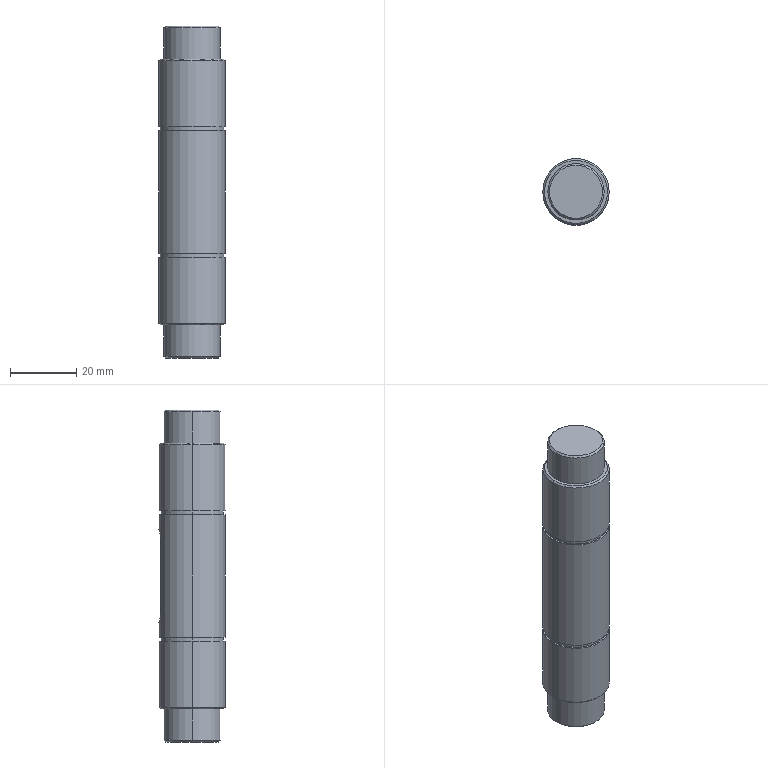Part | SolidWorks | features ICE 3, Chamfer 1, Extrusion 1, MirrorPattern 1 | 1 solid | 36 faces | box 20 x 20 x 100 mm | volume 29039 mm3 | cylinder 17 | plane 11 | cone 8 | commonest cylinder face diameters 20 x6 17 x4 19 x4 6 x3
STEP:
#1=CARTESIAN_POINT('',(0.,6.5,14.));
#2=VERTEX_POINT('',#1);
#3=CARTESIAN_POINT('',(3.,6.5,11.));
#4=VERTEX_POINT('',#3);
#5=CARTESIAN_POINT('',(0.,6.5,11.));
#6=DIRECTION('',(0.,1.,0.));
#7=DIRECTION('',(0.,0.,1.));
#8=AXIS2_PLACEMENT_3D('',#5,#6,#7);
#9=CIRCLE('',#8,3.);
#10=EDGE_CURVE('',#2,#4,#9,.T.);
#11=ORIENTED_EDGE('',*,*,#10,.F.);
#12=CARTESIAN_POINT('',(0.,10.,14.));
#13=VERTEX_POINT('',#12);
#14=CARTESIAN_POINT('',(0.,6.5,14.));
#15=DIRECTION('',(0.,1.,0.));
#16=VECTOR('',#15,1000.);
#17=LINE('',#14,#16);
#18=EDGE_CURVE('',#2,#13,#17,.T.);
#19=ORIENTED_EDGE('',*,*,#18,.T.);
#20=CARTESIAN_POINT('',(3.,9.539,11.));
#21=VERTEX_POINT('',#20);
#22=CARTESIAN_POINT('',(3.,9.539,11.));
#23=CARTESIAN_POINT('',(3.,9.539,11.198));
#24=CARTESIAN_POINT('',(2.981,9.546,11.393));
#25=CARTESIAN_POINT('',(2.904,9.569,11.78));
#26=CARTESIAN_POINT('',(2.845,9.587,11.971));
#27=CARTESIAN_POINT('',(2.62,9.652,12.513));
#28=CARTESIAN_POINT('',(2.397,9.713,12.845));
#29=CARTESIAN_POINT('',(1.985,9.802,13.258));
#30=CARTESIAN_POINT('',(1.832,9.832,13.384));
#31=CARTESIAN_POINT('',(1.506,9.887,13.602));
#32=CARTESIAN_POINT('',(1.335,9.912,13.694));
#33=CARTESIAN_POINT('',(0.973,9.954,13.845));
#34=CARTESIAN_POINT('',(0.7814,9.971,13.903));
#35=CARTESIAN_POINT('',(0.3955,9.994,13.98));
#36=CARTESIAN_POINT('',(0.1994,10.,14.));
#37=CARTESIAN_POINT('',(0.,10.,14.));
#38=B_SPLINE_CURVE_WITH_KNOTS('',3,(#22,#23,#24,#25,#26,#27,#28,#29,#30,#31,#32,#33,#34,#35,#36,#37),.UNSPECIFIED.,.F.,.F.,(4,2,2,2,2,2,2,4),(0.01415,0.01474,0.01533,0.01651,0.0171,0.01769,0.01828,0.01887),.UNSPECIFIED.);
#39=EDGE_CURVE('',#21,#13,#38,.T.);
#40=ORIENTED_EDGE('',*,*,#39,.F.);
#41=CARTESIAN_POINT('',(3.,6.5,11.));
#42=DIRECTION('',(0.,1.,0.));
#43=VECTOR('',#42,1000.);
#44=LINE('',#41,#43);
#45=EDGE_CURVE('',#4,#21,#44,.T.);
#46=ORIENTED_EDGE('',*,*,#45,.F.);
#47=EDGE_LOOP('',(#11,#19,#40,#46));
#48=FACE_OUTER_BOUND('',#47,.T.);
#49=CARTESIAN_POINT('',(0.,6.5,11.));
#50=DIRECTION('',(0.,1.,0.));
#51=DIRECTION('',(0.,0.,1.));
#52=AXIS2_PLACEMENT_3D('',#49,#50,#51);
#53=CYLINDRICAL_SURFACE('',#52,3.);
#54=ADVANCED_FACE('',(#48),#53,.F.);
#55=CARTESIAN_POINT('',(8.,0.,50.));
#56=VERTEX_POINT('',#55);
#57=CARTESIAN_POINT('',(-8.,0.,50.));
#58=VERTEX_POINT('',#57);
#59=CARTESIAN_POINT('',(0.,0.,50.));
#60=DIRECTION('',(0.,0.,1.));
#61=DIRECTION('',(1.,0.,0.));
#62=AXIS2_PLACEMENT_3D('',#59,#60,#61);
#63=CIRCLE('',#62,8.);
#64=EDGE_CURVE('',#56,#58,#63,.T.);
#65=ORIENTED_EDGE('',*,*,#64,.F.);
#66=CARTESIAN_POINT('',(8.5,0.,49.5));
#67=VERTEX_POINT('',#66);
#68=CARTESIAN_POINT('',(8.,0.,50.));
#69=DIRECTION('',(0.7071,0.,-0.7071));
#70=VECTOR('',#69,1000.);
#71=LINE('',#68,#70);
#72=EDGE_CURVE('',#56,#67,#71,.T.);
#73=ORIENTED_EDGE('',*,*,#72,.T.);
#74=CARTESIAN_POINT('',(-8.5,0.,49.5));
#75=VERTEX_POINT('',#74);
#76=CARTESIAN_POINT('',(0.,0.,49.5));
#77=DIRECTION('',(0.,0.,-1.));
#78=DIRECTION('',(1.,0.,0.));
#79=AXIS2_PLACEMENT_3D('',#76,#77,#78);
#80=CIRCLE('',#79,8.5);
#81=EDGE_CURVE('',#75,#67,#80,.T.);
#82=ORIENTED_EDGE('',*,*,#81,.F.);
#83=CARTESIAN_POINT('',(-8.,0.,50.));
#84=DIRECTION('',(-0.7071,0.,-0.7071));
#85=VECTOR('',#84,1000.);
#86=LINE('',#83,#85);
#87=EDGE_CURVE('',#58,#75,#86,.T.);
#88=ORIENTED_EDGE('',*,*,#87,.F.);
#89=EDGE_LOOP('',(#65,#73,#82,#88));
#90=FACE_OUTER_BOUND('',#89,.T.);
#91=CARTESIAN_POINT('',(0.,0.,50.));
#92=DIRECTION('',(0.,0.,-1.));
#93=DIRECTION('',(-1.,0.,0.));
#94=AXIS2_PLACEMENT_3D('',#91,#92,#93);
#95=CONICAL_SURFACE('',#94,8.,0.7854);
#96=ADVANCED_FACE('',(#90),#95,.T.);
#97=CARTESIAN_POINT('',(9.5,0.,40.));
#98=VERTEX_POINT('',#97);
#99=CARTESIAN_POINT('',(-9.5,0.,40.));
#100=VERTEX_POINT('',#99);
#101=CARTESIAN_POINT('',(0.,0.,40.));
#102=DIRECTION('',(0.,0.,1.));
#103=DIRECTION('',(1.,0.,0.));
#104=AXIS2_PLACEMENT_3D('',#101,#102,#103);
#105=CIRCLE('',#104,9.5);
#106=EDGE_CURVE('',#98,#100,#105,.T.);
#107=ORIENTED_EDGE('',*,*,#106,.F.);
#108=CARTESIAN_POINT('',(10.,0.,39.5));
#109=VERTEX_POINT('',#108);
#110=CARTESIAN_POINT('',(9.5,0.,40.));
#111=DIRECTION('',(0.7071,0.,-0.7071));
#112=VECTOR('',#111,1000.);
#113=LINE('',#110,#112);
#114=EDGE_CURVE('',#98,#109,#113,.T.);
#115=ORIENTED_EDGE('',*,*,#114,.T.);
#116=CARTESIAN_POINT('',(-10.,0.,39.5));
#117=VERTEX_POINT('',#116);
#118=CARTESIAN_POINT('',(0.,0.,39.5));
#119=DIRECTION('',(0.,0.,-1.));
#120=DIRECTION('',(1.,0.,0.));
#121=AXIS2_PLACEMENT_3D('',#118,#119,#120);
#122=CIRCLE('',#121,10.);
#123=EDGE_CURVE('',#117,#109,#122,.T.);
#124=ORIENTED_EDGE('',*,*,#123,.F.);
#125=CARTESIAN_POINT('',(-9.5,0.,40.));
#126=DIRECTION('',(-0.7071,0.,-0.7071));
#127=VECTOR('',#126,1000.);
#128=LINE('',#125,#127);
#129=EDGE_CURVE('',#100,#117,#128,.T.);
#130=ORIENTED_EDGE('',*,*,#129,.F.);
#131=EDGE_LOOP('',(#107,#115,#124,#130));
#132=FACE_OUTER_BOUND('',#131,.T.);
#133=CARTESIAN_POINT('',(0.,0.,40.));
#134=DIRECTION('',(0.,0.,-1.));
#135=DIRECTION('',(-1.,0.,0.));
#136=AXIS2_PLACEMENT_3D('',#133,#134,#135);
#137=CONICAL_SURFACE('',#136,9.5,0.7854);
#138=ADVANCED_FACE('',(#132),#137,.T.);
#139=CARTESIAN_POINT('',(-8.,0.,-50.));
#140=VERTEX_POINT('',#139);
#141=CARTESIAN_POINT('',(8.,0.,-50.));
#142=VERTEX_POINT('',#141);
#143=CARTESIAN_POINT('',(0.,0.,-50.));
#144=DIRECTION('',(0.,0.,-1.));
#145=DIRECTION('',(-1.,0.,0.));
#146=AXIS2_PLACEMENT_3D('',#143,#144,#145);
#147=CIRCLE('',#146,8.);
#148=EDGE_CURVE('',#140,#142,#147,.T.);
#149=ORIENTED_EDGE('',*,*,#148,.F.);
#150=CARTESIAN_POINT('',(-8.5,0.,-49.5));
#151=VERTEX_POINT('',#150);
#152=CARTESIAN_POINT('',(-8.5,0.,-49.5));
#153=DIRECTION('',(-0.7071,0.,0.7071));
#154=VECTOR('',#153,1000.);
#155=LINE('',#152,#154);
#156=EDGE_CURVE('',#140,#151,#155,.T.);
#157=ORIENTED_EDGE('',*,*,#156,.T.);
#158=CARTESIAN_POINT('',(8.5,0.,-49.5));
#159=VERTEX_POINT('',#158);
#160=CARTESIAN_POINT('',(0.,0.,-49.5));
#161=DIRECTION('',(0.,0.,1.));
#162=DIRECTION('',(-1.,0.,0.));
#163=AXIS2_PLACEMENT_3D('',#160,#161,#162);
#164=CIRCLE('',#163,8.5);
#165=EDGE_CURVE('',#159,#151,#164,.T.);
#166=ORIENTED_EDGE('',*,*,#165,.F.);
#167=CARTESIAN_POINT('',(8.5,0.,-49.5));
#168=DIRECTION('',(0.7071,0.,0.7071));
#169=VECTOR('',#168,1000.);
#170=LINE('',#167,#169);
#171=EDGE_CURVE('',#142,#159,#170,.T.);
#172=ORIENTED_EDGE('',*,*,#171,.F.);
#173=EDGE_LOOP('',(#149,#157,#166,#172));
#174=FACE_OUTER_BOUND('',#173,.T.);
#175=CARTESIAN_POINT('',(0.,0.,-49.5));
#176=DIRECTION('',(0.,0.,1.));
#177=DIRECTION('',(1.,0.,0.));
#178=AXIS2_PLACEMENT_3D('',#175,#176,#177);
#179=CONICAL_SURFACE('',#178,8.5,0.7854);
#180=ADVANCED_FACE('',(#174),#179,.T.);
#181=CARTESIAN_POINT('',(-9.5,0.,-40.));
#182=VERTEX_POINT('',#181);
#183=CARTESIAN_POINT('',(9.5,0.,-40.));
#184=VERTEX_POINT('',#183);
#185=CARTESIAN_POINT('',(0.,0.,-40.));
#186=DIRECTION('',(0.,0.,-1.));
#187=DIRECTION('',(1.,0.,0.));
#188=AXIS2_PLACEMENT_3D('',#185,#186,#187);
#189=CIRCLE('',#188,9.5);
#190=EDGE_CURVE('',#182,#184,#189,.T.);
#191=ORIENTED_EDGE('',*,*,#190,.F.);
#192=CARTESIAN_POINT('',(-10.,0.,-39.5));
#193=VERTEX_POINT('',#192);
#194=CARTESIAN_POINT('',(-10.,0.,-39.5));
#195=DIRECTION('',(-0.7071,0.,0.7071));
#196=VECTOR('',#195,1000.);
#197=LINE('',#194,#196);
#198=EDGE_CURVE('',#182,#193,#197,.T.);
#199=ORIENTED_EDGE('',*,*,#198,.T.);
#200=CARTESIAN_POINT('',(10.,0.,-39.5));
#201=VERTEX_POINT('',#200);
#202=CARTESIAN_POINT('',(0.,0.,-39.5));
#203=DIRECTION('',(0.,0.,1.));
#204=DIRECTION('',(1.,0.,0.));
#205=AXIS2_PLACEMENT_3D('',#202,#203,#204);
#206=CIRCLE('',#205,10.);
#207=EDGE_CURVE('',#201,#193,#206,.T.);
#208=ORIENTED_EDGE('',*,*,#207,.F.);
#209=CARTESIAN_POINT('',(10.,0.,-39.5));
#210=DIRECTION('',(0.7071,0.,0.7071));
#211=VECTOR('',#210,1000.);
#212=LINE('',#209,#211);
#213=EDGE_CURVE('',#184,#201,#212,.T.);
#214=ORIENTED_EDGE('',*,*,#213,.F.);
#215=EDGE_LOOP('',(#191,#199,#208,#214));
#216=FACE_OUTER_BOUND('',#215,.T.);
#217=CARTESIAN_POINT('',(0.,0.,-39.5));
#218=DIRECTION('',(0.,0.,1.));
#219=DIRECTION('',(1.,0.,0.));
#220=AXIS2_PLACEMENT_3D('',#217,#218,#219);
#221=CONICAL_SURFACE('',#220,10.,0.7854);
#222=ADVANCED_FACE('',(#216),#221,.T.);
#223=CARTESIAN_POINT('',(10.,0.,-19.6));
#224=VERTEX_POINT('',#223);
#225=CARTESIAN_POINT('',(-10.,0.,-19.6));
#226=VERTEX_POINT('',#225);
#227=CARTESIAN_POINT('',(0.,0.,-19.6));
#228=DIRECTION('',(0.,0.,1.));
#229=DIRECTION('',(1.,0.,0.));
#230=AXIS2_PLACEMENT_3D('',#227,#228,#229);
#231=CIRCLE('',#230,10.);
#232=EDGE_CURVE('',#224,#226,#231,.T.);
#233=ORIENTED_EDGE('',*,*,#232,.F.);
#234=CARTESIAN_POINT('',(10.,0.,40.));
#235=DIRECTION('',(0.,0.,-1.));
#236=VECTOR('',#235,1000.);
#237=LINE('',#234,#236);
#238=EDGE_CURVE('',#224,#201,#237,.T.);
#239=ORIENTED_EDGE('',*,*,#238,.T.);
#240=ORIENTED_EDGE('',*,*,#207,.T.);
#241=CARTESIAN_POINT('',(-10.,0.,40.));
#242=DIRECTION('',(0.,0.,-1.));
#243=VECTOR('',#242,1000.);
#244=LINE('',#241,#243);
#245=EDGE_CURVE('',#226,#193,#244,.T.);
#246=ORIENTED_EDGE('',*,*,#245,.F.);
#247=EDGE_LOOP('',(#233,#239,#240,#246));
#248=FACE_OUTER_BOUND('',#247,.T.);
#249=CARTESIAN_POINT('',(0.,0.,40.));
#250=DIRECTION('',(0.,0.,-1.));
#251=DIRECTION('',(-1.,0.,0.));
#252=AXIS2_PLACEMENT_3D('',#249,#250,#251);
#253=CYLINDRICAL_SURFACE('',#252,10.);
#254=ADVANCED_FACE('',(#248),#253,.T.);
#255=ORIENTED_EDGE('',*,*,#165,.T.);
#256=CARTESIAN_POINT('',(-8.5,0.,-40.));
#257=VERTEX_POINT('',#256);
#258=CARTESIAN_POINT('',(-8.5,0.,-50.));
#259=DIRECTION('',(0.,0.,1.));
#260=VECTOR('',#259,1000.);
#261=LINE('',#258,#260);
#262=EDGE_CURVE('',#151,#257,#261,.T.);
#263=ORIENTED_EDGE('',*,*,#262,.T.);
#264=CARTESIAN_POINT('',(8.5,0.,-40.));
#265=VERTEX_POINT('',#264);
#266=CARTESIAN_POINT('',(0.,0.,-40.));
#267=DIRECTION('',(0.,0.,1.));
#268=DIRECTION('',(1.,0.,0.));
#269=AXIS2_PLACEMENT_3D('',#266,#267,#268);
#270=CIRCLE('',#269,8.5);
#271=EDGE_CURVE('',#265,#257,#270,.T.);
#272=ORIENTED_EDGE('',*,*,#271,.F.);
#273=CARTESIAN_POINT('',(8.5,0.,-50.));
#274=DIRECTION('',(0.,0.,1.));
#275=VECTOR('',#274,1000.);
#276=LINE('',#273,#275);
#277=EDGE_CURVE('',#159,#265,#276,.T.);
#278=ORIENTED_EDGE('',*,*,#277,.F.);
#279=EDGE_LOOP('',(#255,#263,#272,#278));
#280=FACE_OUTER_BOUND('',#279,.T.);
#281=CARTESIAN_POINT('',(0.,0.,-50.));
#282=DIRECTION('',(0.,0.,1.));
#283=DIRECTION('',(1.,0.,0.));
#284=AXIS2_PLACEMENT_3D('',#281,#282,#283);
#285=CYLINDRICAL_SURFACE('',#284,8.5);
#286=ADVANCED_FACE('',(#280),#285,.T.);
#287=CARTESIAN_POINT('',(9.5,0.,-19.6));
#288=VERTEX_POINT('',#287);
#289=CARTESIAN_POINT('',(-9.5,0.,-19.6));
#290=VERTEX_POINT('',#289);
#291=CARTESIAN_POINT('',(0.,0.,-19.6));
#292=DIRECTION('',(0.,0.,1.));
#293=DIRECTION('',(1.,0.,0.));
#294=AXIS2_PLACEMENT_3D('',#291,#292,#293);
#295=CIRCLE('',#294,9.5);
#296=EDGE_CURVE('',#288,#290,#295,.T.);
#297=ORIENTED_EDGE('',*,*,#296,.T.);
#298=CARTESIAN_POINT('',(-9.5,0.,-18.5));
#299=VERTEX_POINT('',#298);
#300=CARTESIAN_POINT('',(-9.5,0.,-19.6));
#301=DIRECTION('',(0.,0.,1.));
#302=VECTOR('',#301,1000.);
#303=LINE('',#300,#302);
#304=EDGE_CURVE('',#290,#299,#303,.T.);
#305=ORIENTED_EDGE('',*,*,#304,.T.);
#306=CARTESIAN_POINT('',(9.5,0.,-18.5));
#307=VERTEX_POINT('',#306);
#308=CARTESIAN_POINT('',(0.,0.,-18.5));
#309=DIRECTION('',(0.,0.,1.));
#310=DIRECTION('',(1.,0.,0.));
#311=AXIS2_PLACEMENT_3D('',#308,#309,#310);
#312=CIRCLE('',#311,9.5);
#313=EDGE_CURVE('',#307,#299,#312,.T.);
#314=ORIENTED_EDGE('',*,*,#313,.F.);
#315=CARTESIAN_POINT('',(9.5,0.,-19.6));
#316=DIRECTION('',(0.,0.,1.));
#317=VECTOR('',#316,1000.);
#318=LINE('',#315,#317);
#319=EDGE_CURVE('',#288,#307,#318,.T.);
#320=ORIENTED_EDGE('',*,*,#319,.F.);
#321=EDGE_LOOP('',(#297,#305,#314,#320));
#322=FACE_OUTER_BOUND('',#321,.T.);
#323=CARTESIAN_POINT('',(0.,0.,-19.6));
#324=DIRECTION('',(0.,0.,1.));
#325=DIRECTION('',(1.,0.,0.));
#326=AXIS2_PLACEMENT_3D('',#323,#324,#325);
#327=CYLINDRICAL_SURFACE('',#326,9.5);
#328=ADVANCED_FACE('',(#322),#327,.T.);
#329=CARTESIAN_POINT('',(9.5,0.,19.6));
#330=VERTEX_POINT('',#329);
#331=CARTESIAN_POINT('',(-9.5,0.,19.6));
#332=VERTEX_POINT('',#331);
#333=CARTESIAN_POINT('',(0.,0.,19.6));
#334=DIRECTION('',(0.,0.,1.));
#335=DIRECTION('',(1.,0.,0.));
#336=AXIS2_PLACEMENT_3D('',#333,#334,#335);
#337=CIRCLE('',#336,9.5);
#338=EDGE_CURVE('',#330,#332,#337,.T.);
#339=ORIENTED_EDGE('',*,*,#338,.F.);
#340=CARTESIAN_POINT('',(9.5,0.,18.5));
#341=VERTEX_POINT('',#340);
#342=CARTESIAN_POINT('',(9.5,0.,19.6));
#343=DIRECTION('',(0.,0.,-1.));
#344=VECTOR('',#343,1000.);
#345=LINE('',#342,#344);
#346=EDGE_CURVE('',#330,#341,#345,.T.);
#347=ORIENTED_EDGE('',*,*,#346,.T.);
#348=CARTESIAN_POINT('',(-9.5,0.,18.5));
#349=VERTEX_POINT('',#348);
#350=CARTESIAN_POINT('',(0.,0.,18.5));
#351=DIRECTION('',(0.,0.,1.));
#352=DIRECTION('',(1.,0.,0.));
#353=AXIS2_PLACEMENT_3D('',#350,#351,#352);
#354=CIRCLE('',#353,9.5);
#355=EDGE_CURVE('',#341,#349,#354,.T.);
#356=ORIENTED_EDGE('',*,*,#355,.T.);
#357=CARTESIAN_POINT('',(-9.5,0.,19.6));
#358=DIRECTION('',(0.,0.,-1.));
#359=VECTOR('',#358,1000.);
#360=LINE('',#357,#359);
#361=EDGE_CURVE('',#332,#349,#360,.T.);
#362=ORIENTED_EDGE('',*,*,#361,.F.);
#363=EDGE_LOOP('',(#339,#347,#356,#362));
#364=FACE_OUTER_BOUND('',#363,.T.);
#365=CARTESIAN_POINT('',(0.,0.,19.6));
#366=DIRECTION('',(0.,0.,-1.));
#367=DIRECTION('',(-1.,0.,0.));
#368=AXIS2_PLACEMENT_3D('',#365,#366,#367);
#369=CYLINDRICAL_SURFACE('',#368,9.5);
#370=ADVANCED_FACE('',(#364),#369,.T.);
#371=ORIENTED_EDGE('',*,*,#81,.T.);
#372=CARTESIAN_POINT('',(8.5,0.,40.));
#373=VERTEX_POINT('',#372);
#374=CARTESIAN_POINT('',(8.5,0.,50.));
#375=DIRECTION('',(0.,0.,-1.));
#376=VECTOR('',#375,1000.);
#377=LINE('',#374,#376);
#378=EDGE_CURVE('',#67,#373,#377,.T.);
#379=ORIENTED_EDGE('',*,*,#378,.T.);
#380=CARTESIAN_POINT('',(-8.5,0.,40.));
#381=VERTEX_POINT('',#380);
#382=CARTESIAN_POINT('',(0.,0.,40.));
#383=DIRECTION('',(0.,0.,1.));
#384=DIRECTION('',(1.,0.,0.));
#385=AXIS2_PLACEMENT_3D('',#382,#383,#384);
#386=CIRCLE('',#385,8.5);
#387=EDGE_CURVE('',#373,#381,#386,.T.);
#388=ORIENTED_EDGE('',*,*,#387,.T.);
#389=CARTESIAN_POINT('',(-8.5,0.,50.));
#390=DIRECTION('',(0.,0.,-1.));
#391=VECTOR('',#390,1000.);
#392=LINE('',#389,#391);
#393=EDGE_CURVE('',#75,#381,#392,.T.);
#394=ORIENTED_EDGE('',*,*,#393,.F.);
#395=EDGE_LOOP('',(#371,#379,#388,#394));
#396=FACE_OUTER_BOUND('',#395,.T.);
#397=CARTESIAN_POINT('',(0.,0.,50.));
#398=DIRECTION('',(0.,0.,-1.));
#399=DIRECTION('',(-1.,0.,0.));
#400=AXIS2_PLACEMENT_3D('',#397,#398,#399);
#401=CYLINDRICAL_SURFACE('',#400,8.5);
#402=ADVANCED_FACE('',(#396),#401,.T.);
#403=ORIENTED_EDGE('',*,*,#123,.T.);
#404=CARTESIAN_POINT('',(10.,0.,19.6));
#405=VERTEX_POINT('',#404);
#406=CARTESIAN_POINT('',(10.,0.,40.));
#407=DIRECTION('',(0.,0.,-1.));
#408=VECTOR('',#407,1000.);
#409=LINE('',#406,#408);
#410=EDGE_CURVE('',#109,#405,#409,.T.);
#411=ORIENTED_EDGE('',*,*,#410,.T.);
#412=CARTESIAN_POINT('',(-10.,0.,19.6));
#413=VERTEX_POINT('',#412);
#414=CARTESIAN_POINT('',(0.,0.,19.6));
#415=DIRECTION('',(0.,0.,1.));
#416=DIRECTION('',(1.,0.,0.));
#417=AXIS2_PLACEMENT_3D('',#414,#415,#416);
#418=CIRCLE('',#417,10.);
#419=EDGE_CURVE('',#405,#413,#418,.T.);
#420=ORIENTED_EDGE('',*,*,#419,.T.);
#421=CARTESIAN_POINT('',(-10.,0.,40.));
#422=DIRECTION('',(0.,0.,-1.));
#423=VECTOR('',#422,1000.);
#424=LINE('',#421,#423);
#425=EDGE_CURVE('',#117,#413,#424,.T.);
#426=ORIENTED_EDGE('',*,*,#425,.F.);
#427=EDGE_LOOP('',(#403,#411,#420,#426));
#428=FACE_OUTER_BOUND('',#427,.T.);
#429=CARTESIAN_POINT('',(0.,0.,40.));
#430=DIRECTION('',(0.,0.,-1.));
#431=DIRECTION('',(-1.,0.,0.));
#432=AXIS2_PLACEMENT_3D('',#429,#430,#431);
#433=CYLINDRICAL_SURFACE('',#432,10.);
#434=ADVANCED_FACE('',(#428),#433,.T.);
#435=ORIENTED_EDGE('',*,*,#39,.T.);
#436=CARTESIAN_POINT('',(-3.,9.539,11.));
#437=VERTEX_POINT('',#436);
#438=CARTESIAN_POINT('',(0.,10.,14.));
#439=CARTESIAN_POINT('',(-0.1995,10.,14.));
#440=CARTESIAN_POINT('',(-0.3955,9.994,13.98));
#441=CARTESIAN_POINT('',(-0.7806,9.971,13.903));
#442=CARTESIAN_POINT('',(-0.9719,9.954,13.845));
#443=CARTESIAN_POINT('',(-1.335,9.912,13.694));
#444=CARTESIAN_POINT('',(-1.507,9.887,13.602));
#445=CARTESIAN_POINT('',(-1.832,9.832,13.384));
#446=CARTESIAN_POINT('',(-1.985,9.802,13.258));
#447=CARTESIAN_POINT('',(-2.398,9.712,12.845));
#448=CARTESIAN_POINT('',(-2.62,9.652,12.512));
#449=CARTESIAN_POINT('',(-2.845,9.587,11.971));
#450=CARTESIAN_POINT('',(-2.903,9.569,11.78));
#451=CARTESIAN_POINT('',(-2.981,9.546,11.393));
#452=CARTESIAN_POINT('',(-3.,9.539,11.197));
#453=CARTESIAN_POINT('',(-3.,9.539,11.));
#454=B_SPLINE_CURVE_WITH_KNOTS('',3,(#438,#439,#440,#441,#442,#443,#444,#445,#446,#447,#448,#449,#450,#451,#452,#453),.UNSPECIFIED.,.F.,.F.,(4,2,2,2,2,2,2,4),(0.,0.0005898,0.00118,0.001769,0.002359,0.003539,0.004129,0.004718),.UNSPECIFIED.);
#455=EDGE_CURVE('',#13,#437,#454,.T.);
#456=ORIENTED_EDGE('',*,*,#455,.T.);
#457=CARTESIAN_POINT('',(-3.,9.539,-11.));
#458=VERTEX_POINT('',#457);
#459=CARTESIAN_POINT('',(-3.,9.539,40.));
#460=DIRECTION('',(0.,0.,-1.));
#461=VECTOR('',#460,1000.);
#462=LINE('',#459,#461);
#463=EDGE_CURVE('',#437,#458,#462,.T.);
#464=ORIENTED_EDGE('',*,*,#463,.T.);
#465=CARTESIAN_POINT('',(3.,9.539,-11.));
#466=VERTEX_POINT('',#465);
#467=CARTESIAN_POINT('',(-3.,9.539,-11.));
#468=CARTESIAN_POINT('',(-3.,9.539,-11.199));
#469=CARTESIAN_POINT('',(-2.98,9.546,-11.395));
#470=CARTESIAN_POINT('',(-2.903,9.569,-11.78));
#471=CARTESIAN_POINT('',(-2.845,9.587,-11.971));
#472=CARTESIAN_POINT('',(-2.694,9.631,-12.334));
#473=CARTESIAN_POINT('',(-2.602,9.656,-12.506));
#474=CARTESIAN_POINT('',(-2.385,9.712,-12.831));
#475=CARTESIAN_POINT('',(-2.259,9.743,-12.984));
#476=CARTESIAN_POINT('',(-1.847,9.832,-13.396));
#477=CARTESIAN_POINT('',(-1.514,9.891,-13.619));
#478=CARTESIAN_POINT('',(-0.9732,9.954,-13.844));
#479=CARTESIAN_POINT('',(-0.783,9.971,-13.903));
#480=CARTESIAN_POINT('',(-0.3953,9.994,-13.98));
#481=CARTESIAN_POINT('',(-0.1999,10.,-14.));
#482=CARTESIAN_POINT('',(0.194,10.,-14.));
#483=CARTESIAN_POINT('',(0.394,9.994,-13.981));
#484=CARTESIAN_POINT('',(0.7797,9.971,-13.904));
#485=CARTESIAN_POINT('',(0.9673,9.955,-13.847));
#486=CARTESIAN_POINT('',(1.332,9.913,-13.695));
#487=CARTESIAN_POINT('',(1.506,9.887,-13.602));
#488=CARTESIAN_POINT('',(1.83,9.833,-13.386));
#489=CARTESIAN_POINT('',(1.982,9.803,-13.26));
#490=CARTESIAN_POINT('',(2.259,9.743,-12.984));
#491=CARTESIAN_POINT('',(2.383,9.713,-12.833));
#492=CARTESIAN_POINT('',(2.6,9.657,-12.51));
#493=CARTESIAN_POINT('',(2.694,9.631,-12.334));
#494=CARTESIAN_POINT('',(2.845,9.587,-11.973));
#495=CARTESIAN_POINT('',(2.902,9.57,-11.786));
#496=CARTESIAN_POINT('',(2.98,9.546,-11.399));
#497=CARTESIAN_POINT('',(3.,9.539,-11.199));
#498=CARTESIAN_POINT('',(3.,9.539,-11.));
#499=B_SPLINE_CURVE_WITH_KNOTS('',3,(#467,#468,#469,#470,#471,#472,#473,#474,#475,#476,#477,#478,#479,#480,#481,#482,#483,#484,#485,#486,#487,#488,#489,#490,#491,#492,#493,#494,#495,#496,#497,#498),.UNSPECIFIED.,.F.,.F.,(4,2,2,2,2,2,2,2,2,2,2,2,2,2,2,4),(0.,0.0005894,0.001179,0.001768,0.002358,0.003536,0.004126,0.004715,0.005305,0.005894,0.006484,0.007073,0.007662,0.008252,0.008841,0.009431),.UNSPECIFIED.);
#500=EDGE_CURVE('',#458,#466,#499,.T.);
#501=ORIENTED_EDGE('',*,*,#500,.T.);
#502=CARTESIAN_POINT('',(3.,9.539,40.));
#503=DIRECTION('',(0.,0.,1.));
#504=VECTOR('',#503,1000.);
#505=LINE('',#502,#504);
#506=EDGE_CURVE('',#466,#21,#505,.T.);
#507=ORIENTED_EDGE('',*,*,#506,.T.);
#508=EDGE_LOOP('',(#435,#456,#464,#501,#507));
#509=FACE_BOUND('',#508,.T.);
#510=CARTESIAN_POINT('',(10.,0.,18.5));
#511=VERTEX_POINT('',#510);
#512=CARTESIAN_POINT('',(-10.,0.,18.5));
#513=VERTEX_POINT('',#512);
#514=CARTESIAN_POINT('',(0.,0.,18.5));
#515=DIRECTION('',(0.,0.,1.));
#516=DIRECTION('',(1.,0.,0.));
#517=AXIS2_PLACEMENT_3D('',#514,#515,#516);
#518=CIRCLE('',#517,10.);
#519=EDGE_CURVE('',#511,#513,#518,.T.);
#520=ORIENTED_EDGE('',*,*,#519,.F.);
#521=CARTESIAN_POINT('',(10.,0.,-18.5));
#522=VERTEX_POINT('',#521);
#523=CARTESIAN_POINT('',(10.,0.,40.));
#524=DIRECTION('',(0.,0.,-1.));
#525=VECTOR('',#524,1000.);
#526=LINE('',#523,#525);
#527=EDGE_CURVE('',#511,#522,#526,.T.);
#528=ORIENTED_EDGE('',*,*,#527,.T.);
#529=CARTESIAN_POINT('',(-10.,0.,-18.5));
#530=VERTEX_POINT('',#529);
#531=CARTESIAN_POINT('',(0.,0.,-18.5));
#532=DIRECTION('',(0.,0.,1.));
#533=DIRECTION('',(1.,0.,0.));
#534=AXIS2_PLACEMENT_3D('',#531,#532,#533);
#535=CIRCLE('',#534,10.);
#536=EDGE_CURVE('',#522,#530,#535,.T.);
#537=ORIENTED_EDGE('',*,*,#536,.T.);
#538=CARTESIAN_POINT('',(-10.,0.,40.));
#539=DIRECTION('',(0.,0.,-1.));
#540=VECTOR('',#539,1000.);
#541=LINE('',#538,#540);
#542=EDGE_CURVE('',#513,#530,#541,.T.);
#543=ORIENTED_EDGE('',*,*,#542,.F.);
#544=EDGE_LOOP('',(#520,#528,#537,#543));
#545=FACE_OUTER_BOUND('',#544,.T.);
#546=CARTESIAN_POINT('',(0.,0.,40.));
#547=DIRECTION('',(0.,0.,-1.));
#548=DIRECTION('',(-1.,0.,0.));
#549=AXIS2_PLACEMENT_3D('',#546,#547,#548);
#550=CYLINDRICAL_SURFACE('',#549,10.);
#551=ADVANCED_FACE('',(#509,#545),#550,.T.);
#552=ORIENTED_EDGE('',*,*,#527,.F.);
#553=CARTESIAN_POINT('',(0.,0.,18.5));
#554=DIRECTION('',(0.,0.,1.));
#555=DIRECTION('',(1.,0.,0.));
#556=AXIS2_PLACEMENT_3D('',#553,#554,#555);
#557=CIRCLE('',#556,10.);
#558=EDGE_CURVE('',#513,#511,#557,.T.);
#559=ORIENTED_EDGE('',*,*,#558,.F.);
#560=ORIENTED_EDGE('',*,*,#542,.T.);
#561=CARTESIAN_POINT('',(0.,0.,-18.5));
#562=DIRECTION('',(0.,0.,1.));
#563=DIRECTION('',(1.,0.,0.));
#564=AXIS2_PLACEMENT_3D('',#561,#562,#563);
#565=CIRCLE('',#564,10.);
#566=EDGE_CURVE('',#530,#522,#565,.T.);
#567=ORIENTED_EDGE('',*,*,#566,.T.);
#568=EDGE_LOOP('',(#552,#559,#560,#567));
#569=FACE_OUTER_BOUND('',#568,.T.);
#570=CARTESIAN_POINT('',(0.,0.,40.));
#571=DIRECTION('',(0.,0.,-1.));
#572=DIRECTION('',(-1.,0.,0.));
#573=AXIS2_PLACEMENT_3D('',#570,#571,#572);
#574=CYLINDRICAL_SURFACE('',#573,10.);
#575=ADVANCED_FACE('',(#569),#574,.T.);
#576=CARTESIAN_POINT('',(0.,0.,40.));
#577=DIRECTION('',(0.,0.,1.));
#578=DIRECTION('',(1.,0.,0.));
#579=AXIS2_PLACEMENT_3D('',#576,#577,#578);
#580=CIRCLE('',#579,9.5);
#581=EDGE_CURVE('',#100,#98,#580,.T.);
#582=ORIENTED_EDGE('',*,*,#581,.T.);
#583=ORIENTED_EDGE('',*,*,#106,.T.);
#584=EDGE_LOOP('',(#582,#583));
#585=FACE_OUTER_BOUND('',#584,.T.);
#586=CARTESIAN_POINT('',(0.,0.,40.));
#587=DIRECTION('',(0.,0.,1.));
#588=DIRECTION('',(1.,0.,0.));
#589=AXIS2_PLACEMENT_3D('',#586,#587,#588);
#590=CIRCLE('',#589,8.5);
#591=EDGE_CURVE('',#381,#373,#590,.T.);
#592=ORIENTED_EDGE('',*,*,#591,.F.);
#593=ORIENTED_EDGE('',*,*,#387,.F.);
#594=EDGE_LOOP('',(#592,#593));
#595=FACE_BOUND('',#594,.T.);
#596=CARTESIAN_POINT('',(0.,0.,40.));
#597=DIRECTION('',(0.,0.,1.));
#598=DIRECTION('',(1.,0.,0.));
#599=AXIS2_PLACEMENT_3D('',#596,#597,#598);
#600=PLANE('',#599);
#601=ADVANCED_FACE('',(#585,#595),#600,.T.);
#602=ORIENTED_EDGE('',*,*,#410,.F.);
#603=CARTESIAN_POINT('',(0.,0.,39.5));
#604=DIRECTION('',(0.,0.,-1.));
#605=DIRECTION('',(1.,0.,0.));
#606=AXIS2_PLACEMENT_3D('',#603,#604,#605);
#607=CIRCLE('',#606,10.);
#608=EDGE_CURVE('',#109,#117,#607,.T.);
#609=ORIENTED_EDGE('',*,*,#608,.T.);
#610=ORIENTED_EDGE('',*,*,#425,.T.);
#611=CARTESIAN_POINT('',(0.,0.,19.6));
#612=DIRECTION('',(0.,0.,1.));
#613=DIRECTION('',(1.,0.,0.));
#614=AXIS2_PLACEMENT_3D('',#611,#612,#613);
#615=CIRCLE('',#614,10.);
#616=EDGE_CURVE('',#413,#405,#615,.T.);
#617=ORIENTED_EDGE('',*,*,#616,.T.);
#618=EDGE_LOOP('',(#602,#609,#610,#617));
#619=FACE_OUTER_BOUND('',#618,.T.);
#620=CARTESIAN_POINT('',(0.,0.,40.));
#621=DIRECTION('',(0.,0.,-1.));
#622=DIRECTION('',(-1.,0.,0.));
#623=AXIS2_PLACEMENT_3D('',#620,#621,#622);
#624=CYLINDRICAL_SURFACE('',#623,10.);
#625=ADVANCED_FACE('',(#619),#624,.T.);
#626=ORIENTED_EDGE('',*,*,#378,.F.);
#627=CARTESIAN_POINT('',(0.,0.,49.5));
#628=DIRECTION('',(0.,0.,-1.));
#629=DIRECTION('',(1.,0.,0.));
#630=AXIS2_PLACEMENT_3D('',#627,#628,#629);
#631=CIRCLE('',#630,8.5);
#632=EDGE_CURVE('',#67,#75,#631,.T.);
#633=ORIENTED_EDGE('',*,*,#632,.T.);
#634=ORIENTED_EDGE('',*,*,#393,.T.);
#635=ORIENTED_EDGE('',*,*,#591,.T.);
#636=EDGE_LOOP('',(#626,#633,#634,#635));
#637=FACE_OUTER_BOUND('',#636,.T.);
#638=CARTESIAN_POINT('',(0.,0.,50.));
#639=DIRECTION('',(0.,0.,-1.));
#640=DIRECTION('',(-1.,0.,0.));
#641=AXIS2_PLACEMENT_3D('',#638,#639,#640);
#642=CYLINDRICAL_SURFACE('',#641,8.5);
#643=ADVANCED_FACE('',(#637),#642,.T.);
#644=CARTESIAN_POINT('',(0.,0.,50.));
#645=DIRECTION('',(0.,0.,1.));
#646=DIRECTION('',(1.,0.,0.));
#647=AXIS2_PLACEMENT_3D('',#644,#645,#646);
#648=CIRCLE('',#647,8.);
#649=EDGE_CURVE('',#58,#56,#648,.T.);
#650=ORIENTED_EDGE('',*,*,#649,.T.);
#651=ORIENTED_EDGE('',*,*,#64,.T.);
#652=EDGE_LOOP('',(#650,#651));
#653=FACE_OUTER_BOUND('',#652,.T.);
#654=CARTESIAN_POINT('',(0.,0.,50.));
#655=DIRECTION('',(0.,0.,1.));
#656=DIRECTION('',(1.,0.,0.));
#657=AXIS2_PLACEMENT_3D('',#654,#655,#656);
#658=PLANE('',#657);
#659=ADVANCED_FACE('',(#653),#658,.T.);
#660=ORIENTED_EDGE('',*,*,#616,.F.);
#661=ORIENTED_EDGE('',*,*,#419,.F.);
#662=EDGE_LOOP('',(#660,#661));
#663=FACE_OUTER_BOUND('',#662,.T.);
#664=CARTESIAN_POINT('',(0.,0.,19.6));
#665=DIRECTION('',(0.,0.,1.));
#666=DIRECTION('',(1.,0.,0.));
#667=AXIS2_PLACEMENT_3D('',#664,#665,#666);
#668=CIRCLE('',#667,9.5);
#669=EDGE_CURVE('',#332,#330,#668,.T.);
#670=ORIENTED_EDGE('',*,*,#669,.T.);
#671=ORIENTED_EDGE('',*,*,#338,.T.);
#672=EDGE_LOOP('',(#670,#671));
#673=FACE_BOUND('',#672,.T.);
#674=CARTESIAN_POINT('',(0.,0.,19.6));
#675=DIRECTION('',(0.,0.,1.));
#676=DIRECTION('',(1.,0.,0.));
#677=AXIS2_PLACEMENT_3D('',#674,#675,#676);
#678=PLANE('',#677);
#679=ADVANCED_FACE('',(#663,#673),#678,.F.);
#680=ORIENTED_EDGE('',*,*,#558,.T.);
#681=ORIENTED_EDGE('',*,*,#519,.T.);
#682=EDGE_LOOP('',(#680,#681));
#683=FACE_OUTER_BOUND('',#682,.T.);
#684=CARTESIAN_POINT('',(0.,0.,18.5));
#685=DIRECTION('',(0.,0.,1.));
#686=DIRECTION('',(1.,0.,0.));
#687=AXIS2_PLACEMENT_3D('',#684,#685,#686);
#688=CIRCLE('',#687,9.5);
#689=EDGE_CURVE('',#349,#341,#688,.T.);
#690=ORIENTED_EDGE('',*,*,#689,.F.);
#691=ORIENTED_EDGE('',*,*,#355,.F.);
#692=EDGE_LOOP('',(#690,#691));
#693=FACE_BOUND('',#692,.T.);
#694=CARTESIAN_POINT('',(0.,0.,18.5));
#695=DIRECTION('',(0.,0.,1.));
#696=DIRECTION('',(1.,0.,0.));
#697=AXIS2_PLACEMENT_3D('',#694,#695,#696);
#698=PLANE('',#697);
#699=ADVANCED_FACE('',(#683,#693),#698,.T.);
#700=ORIENTED_EDGE('',*,*,#346,.F.);
#701=ORIENTED_EDGE('',*,*,#669,.F.);
#702=ORIENTED_EDGE('',*,*,#361,.T.);
#703=ORIENTED_EDGE('',*,*,#689,.T.);
#704=EDGE_LOOP('',(#700,#701,#702,#703));
#705=FACE_OUTER_BOUND('',#704,.T.);
#706=CARTESIAN_POINT('',(0.,0.,19.6));
#707=DIRECTION('',(0.,0.,-1.));
#708=DIRECTION('',(-1.,0.,0.));
#709=AXIS2_PLACEMENT_3D('',#706,#707,#708);
#710=CYLINDRICAL_SURFACE('',#709,9.5);
#711=ADVANCED_FACE('',(#705),#710,.T.);
#712=ORIENTED_EDGE('',*,*,#296,.F.);
#713=CARTESIAN_POINT('',(0.,0.,-19.6));
#714=DIRECTION('',(0.,0.,1.));
#715=DIRECTION('',(1.,0.,0.));
#716=AXIS2_PLACEMENT_3D('',#713,#714,#715);
#717=CIRCLE('',#716,9.5);
#718=EDGE_CURVE('',#290,#288,#717,.T.);
#719=ORIENTED_EDGE('',*,*,#718,.F.);
#720=EDGE_LOOP('',(#712,#719));
#721=FACE_BOUND('',#720,.T.);
#722=CARTESIAN_POINT('',(0.,0.,-19.6));
#723=DIRECTION('',(0.,0.,1.));
#724=DIRECTION('',(1.,0.,0.));
#725=AXIS2_PLACEMENT_3D('',#722,#723,#724);
#726=CIRCLE('',#725,10.);
#727=EDGE_CURVE('',#226,#224,#726,.T.);
#728=ORIENTED_EDGE('',*,*,#727,.T.);
#729=ORIENTED_EDGE('',*,*,#232,.T.);
#730=EDGE_LOOP('',(#728,#729));
#731=FACE_OUTER_BOUND('',#730,.T.);
#732=CARTESIAN_POINT('',(0.,0.,-19.6));
#733=DIRECTION('',(0.,0.,-1.));
#734=DIRECTION('',(1.,0.,0.));
#735=AXIS2_PLACEMENT_3D('',#732,#733,#734);
#736=PLANE('',#735);
#737=ADVANCED_FACE('',(#721,#731),#736,.F.);
#738=ORIENTED_EDGE('',*,*,#313,.T.);
#739=CARTESIAN_POINT('',(0.,0.,-18.5));
#740=DIRECTION('',(0.,0.,1.));
#741=DIRECTION('',(1.,0.,0.));
#742=AXIS2_PLACEMENT_3D('',#739,#740,#741);
#743=CIRCLE('',#742,9.5);
#744=EDGE_CURVE('',#299,#307,#743,.T.);
#745=ORIENTED_EDGE('',*,*,#744,.T.);
#746=EDGE_LOOP('',(#738,#745));
#747=FACE_BOUND('',#746,.T.);
#748=ORIENTED_EDGE('',*,*,#566,.F.);
#749=ORIENTED_EDGE('',*,*,#536,.F.);
#750=EDGE_LOOP('',(#748,#749));
#751=FACE_OUTER_BOUND('',#750,.T.);
#752=CARTESIAN_POINT('',(0.,0.,-18.5));
#753=DIRECTION('',(0.,0.,-1.));
#754=DIRECTION('',(1.,0.,0.));
#755=AXIS2_PLACEMENT_3D('',#752,#753,#754);
#756=PLANE('',#755);
#757=ADVANCED_FACE('',(#747,#751),#756,.T.);
#758=ORIENTED_EDGE('',*,*,#304,.F.);
#759=ORIENTED_EDGE('',*,*,#718,.T.);
#760=ORIENTED_EDGE('',*,*,#319,.T.);
#761=ORIENTED_EDGE('',*,*,#744,.F.);
#762=EDGE_LOOP('',(#758,#759,#760,#761));
#763=FACE_OUTER_BOUND('',#762,.T.);
#764=CARTESIAN_POINT('',(0.,0.,-19.6));
#765=DIRECTION('',(0.,0.,1.));
#766=DIRECTION('',(1.,0.,0.));
#767=AXIS2_PLACEMENT_3D('',#764,#765,#766);
#768=CYLINDRICAL_SURFACE('',#767,9.5);
#769=ADVANCED_FACE('',(#763),#768,.T.);
#770=CARTESIAN_POINT('',(0.,0.,-50.));
#771=DIRECTION('',(0.,0.,-1.));
#772=DIRECTION('',(-1.,0.,0.));
#773=AXIS2_PLACEMENT_3D('',#770,#771,#772);
#774=CIRCLE('',#773,8.);
#775=EDGE_CURVE('',#142,#140,#774,.T.);
#776=ORIENTED_EDGE('',*,*,#775,.T.);
#777=ORIENTED_EDGE('',*,*,#148,.T.);
#778=EDGE_LOOP('',(#776,#777));
#779=FACE_OUTER_BOUND('',#778,.T.);
#780=CARTESIAN_POINT('',(0.,0.,-50.));
#781=DIRECTION('',(0.,0.,-1.));
#782=DIRECTION('',(1.,0.,0.));
#783=AXIS2_PLACEMENT_3D('',#780,#781,#782);
#784=PLANE('',#783);
#785=ADVANCED_FACE('',(#779),#784,.T.);
#786=ORIENTED_EDGE('',*,*,#262,.F.);
#787=CARTESIAN_POINT('',(0.,0.,-49.5));
#788=DIRECTION('',(0.,0.,1.));
#789=DIRECTION('',(-1.,0.,0.));
#790=AXIS2_PLACEMENT_3D('',#787,#788,#789);
#791=CIRCLE('',#790,8.5);
#792=EDGE_CURVE('',#151,#159,#791,.T.);
#793=ORIENTED_EDGE('',*,*,#792,.T.);
#794=ORIENTED_EDGE('',*,*,#277,.T.);
#795=CARTESIAN_POINT('',(0.,0.,-40.));
#796=DIRECTION('',(0.,0.,1.));
#797=DIRECTION('',(1.,0.,0.));
#798=AXIS2_PLACEMENT_3D('',#795,#796,#797);
#799=CIRCLE('',#798,8.5);
#800=EDGE_CURVE('',#257,#265,#799,.T.);
#801=ORIENTED_EDGE('',*,*,#800,.F.);
#802=EDGE_LOOP('',(#786,#793,#794,#801));
#803=FACE_OUTER_BOUND('',#802,.T.);
#804=CARTESIAN_POINT('',(0.,0.,-50.));
#805=DIRECTION('',(0.,0.,1.));
#806=DIRECTION('',(1.,0.,0.));
#807=AXIS2_PLACEMENT_3D('',#804,#805,#806);
#808=CYLINDRICAL_SURFACE('',#807,8.5);
#809=ADVANCED_FACE('',(#803),#808,.T.);
#810=CARTESIAN_POINT('',(0.,0.,-40.));
#811=DIRECTION('',(0.,0.,-1.));
#812=DIRECTION('',(1.,0.,0.));
#813=AXIS2_PLACEMENT_3D('',#810,#811,#812);
#814=CIRCLE('',#813,9.5);
#815=EDGE_CURVE('',#184,#182,#814,.T.);
#816=ORIENTED_EDGE('',*,*,#815,.T.);
#817=ORIENTED_EDGE('',*,*,#190,.T.);
#818=EDGE_LOOP('',(#816,#817));
#819=FACE_OUTER_BOUND('',#818,.T.);
#820=ORIENTED_EDGE('',*,*,#271,.T.);
#821=ORIENTED_EDGE('',*,*,#800,.T.);
#822=EDGE_LOOP('',(#820,#821));
#823=FACE_BOUND('',#822,.T.);
#824=CARTESIAN_POINT('',(0.,0.,-40.));
#825=DIRECTION('',(0.,0.,1.));
#826=DIRECTION('',(1.,0.,0.));
#827=AXIS2_PLACEMENT_3D('',#824,#825,#826);
#828=PLANE('',#827);
#829=ADVANCED_FACE('',(#819,#823),#828,.F.);
#830=ORIENTED_EDGE('',*,*,#238,.F.);
#831=ORIENTED_EDGE('',*,*,#727,.F.);
#832=ORIENTED_EDGE('',*,*,#245,.T.);
#833=CARTESIAN_POINT('',(0.,0.,-39.5));
#834=DIRECTION('',(0.,0.,1.));
#835=DIRECTION('',(1.,0.,0.));
#836=AXIS2_PLACEMENT_3D('',#833,#834,#835);
#837=CIRCLE('',#836,10.);
#838=EDGE_CURVE('',#193,#201,#837,.T.);
#839=ORIENTED_EDGE('',*,*,#838,.T.);
#840=EDGE_LOOP('',(#830,#831,#832,#839));
#841=FACE_OUTER_BOUND('',#840,.T.);
#842=CARTESIAN_POINT('',(0.,0.,40.));
#843=DIRECTION('',(0.,0.,-1.));
#844=DIRECTION('',(-1.,0.,0.));
#845=AXIS2_PLACEMENT_3D('',#842,#843,#844);
#846=CYLINDRICAL_SURFACE('',#845,10.);
#847=ADVANCED_FACE('',(#841),#846,.T.);
#848=ORIENTED_EDGE('',*,*,#198,.F.);
#849=ORIENTED_EDGE('',*,*,#815,.F.);
#850=ORIENTED_EDGE('',*,*,#213,.T.);
#851=ORIENTED_EDGE('',*,*,#838,.F.);
#852=EDGE_LOOP('',(#848,#849,#850,#851));
#853=FACE_OUTER_BOUND('',#852,.T.);
#854=CARTESIAN_POINT('',(0.,0.,-39.5));
#855=DIRECTION('',(0.,0.,1.));
#856=DIRECTION('',(1.,0.,0.));
#857=AXIS2_PLACEMENT_3D('',#854,#855,#856);
#858=CONICAL_SURFACE('',#857,10.,0.7854);
#859=ADVANCED_FACE('',(#853),#858,.T.);
#860=ORIENTED_EDGE('',*,*,#156,.F.);
#861=ORIENTED_EDGE('',*,*,#775,.F.);
#862=ORIENTED_EDGE('',*,*,#171,.T.);
#863=ORIENTED_EDGE('',*,*,#792,.F.);
#864=EDGE_LOOP('',(#860,#861,#862,#863));
#865=FACE_OUTER_BOUND('',#864,.T.);
#866=CARTESIAN_POINT('',(0.,0.,-49.5));
#867=DIRECTION('',(0.,0.,1.));
#868=DIRECTION('',(1.,0.,0.));
#869=AXIS2_PLACEMENT_3D('',#866,#867,#868);
#870=CONICAL_SURFACE('',#869,8.5,0.7854);
#871=ADVANCED_FACE('',(#865),#870,.T.);
#872=ORIENTED_EDGE('',*,*,#114,.F.);
#873=ORIENTED_EDGE('',*,*,#581,.F.);
#874=ORIENTED_EDGE('',*,*,#129,.T.);
#875=ORIENTED_EDGE('',*,*,#608,.F.);
#876=EDGE_LOOP('',(#872,#873,#874,#875));
#877=FACE_OUTER_BOUND('',#876,.T.);
#878=CARTESIAN_POINT('',(0.,0.,40.));
#879=DIRECTION('',(0.,0.,-1.));
#880=DIRECTION('',(-1.,0.,0.));
#881=AXIS2_PLACEMENT_3D('',#878,#879,#880);
#882=CONICAL_SURFACE('',#881,9.5,0.7854);
#883=ADVANCED_FACE('',(#877),#882,.T.);
#884=ORIENTED_EDGE('',*,*,#72,.F.);
#885=ORIENTED_EDGE('',*,*,#649,.F.);
#886=ORIENTED_EDGE('',*,*,#87,.T.);
#887=ORIENTED_EDGE('',*,*,#632,.F.);
#888=EDGE_LOOP('',(#884,#885,#886,#887));
#889=FACE_OUTER_BOUND('',#888,.T.);
#890=CARTESIAN_POINT('',(0.,0.,50.));
#891=DIRECTION('',(0.,0.,-1.));
#892=DIRECTION('',(-1.,0.,0.));
#893=AXIS2_PLACEMENT_3D('',#890,#891,#892);
#894=CONICAL_SURFACE('',#893,8.,0.7854);
#895=ADVANCED_FACE('',(#889),#894,.T.);
#896=CARTESIAN_POINT('',(-3.,6.5,-11.));
#897=VERTEX_POINT('',#896);
#898=CARTESIAN_POINT('',(-3.,6.5,-11.));
#899=DIRECTION('',(0.,1.,0.));
#900=VECTOR('',#899,1000.);
#901=LINE('',#898,#900);
#902=EDGE_CURVE('',#897,#458,#901,.T.);
#903=ORIENTED_EDGE('',*,*,#902,.F.);
#904=CARTESIAN_POINT('',(3.,6.5,-11.));
#905=VERTEX_POINT('',#904);
#906=CARTESIAN_POINT('',(0.,6.5,-11.));
#907=DIRECTION('',(0.,1.,0.));
#908=DIRECTION('',(0.,0.,1.));
#909=AXIS2_PLACEMENT_3D('',#906,#907,#908);
#910=CIRCLE('',#909,3.);
#911=EDGE_CURVE('',#905,#897,#910,.T.);
#912=ORIENTED_EDGE('',*,*,#911,.F.);
#913=CARTESIAN_POINT('',(3.,6.5,-11.));
#914=DIRECTION('',(0.,1.,0.));
#915=VECTOR('',#914,1000.);
#916=LINE('',#913,#915);
#917=EDGE_CURVE('',#905,#466,#916,.T.);
#918=ORIENTED_EDGE('',*,*,#917,.T.);
#919=ORIENTED_EDGE('',*,*,#500,.F.);
#920=EDGE_LOOP('',(#903,#912,#918,#919));
#921=FACE_OUTER_BOUND('',#920,.T.);
#922=CARTESIAN_POINT('',(0.,6.5,-11.));
#923=DIRECTION('',(0.,1.,0.));
#924=DIRECTION('',(0.,0.,1.));
#925=AXIS2_PLACEMENT_3D('',#922,#923,#924);
#926=CYLINDRICAL_SURFACE('',#925,3.);
#927=ADVANCED_FACE('',(#921),#926,.F.);
#928=ORIENTED_EDGE('',*,*,#917,.F.);
#929=CARTESIAN_POINT('',(3.,6.5,-11.));
#930=DIRECTION('',(0.,0.,-1.));
#931=VECTOR('',#930,1000.);
#932=LINE('',#929,#931);
#933=EDGE_CURVE('',#4,#905,#932,.T.);
#934=ORIENTED_EDGE('',*,*,#933,.F.);
#935=ORIENTED_EDGE('',*,*,#45,.T.);
#936=ORIENTED_EDGE('',*,*,#506,.F.);
#937=EDGE_LOOP('',(#928,#934,#935,#936));
#938=FACE_OUTER_BOUND('',#937,.T.);
#939=CARTESIAN_POINT('',(3.,6.5,-11.));
#940=DIRECTION('',(1.,0.,0.));
#941=DIRECTION('',(0.,0.,-1.));
#942=AXIS2_PLACEMENT_3D('',#939,#940,#941);
#943=PLANE('',#942);
#944=ADVANCED_FACE('',(#938),#943,.F.);
#945=ORIENTED_EDGE('',*,*,#18,.F.);
#946=CARTESIAN_POINT('',(-3.,6.5,11.));
#947=VERTEX_POINT('',#946);
#948=CARTESIAN_POINT('',(0.,6.5,11.));
#949=DIRECTION('',(0.,1.,0.));
#950=DIRECTION('',(0.,0.,1.));
#951=AXIS2_PLACEMENT_3D('',#948,#949,#950);
#952=CIRCLE('',#951,3.);
#953=EDGE_CURVE('',#947,#2,#952,.T.);
#954=ORIENTED_EDGE('',*,*,#953,.F.);
#955=CARTESIAN_POINT('',(-3.,6.5,11.));
#956=DIRECTION('',(0.,1.,0.));
#957=VECTOR('',#956,1000.);
#958=LINE('',#955,#957);
#959=EDGE_CURVE('',#947,#437,#958,.T.);
#960=ORIENTED_EDGE('',*,*,#959,.T.);
#961=ORIENTED_EDGE('',*,*,#455,.F.);
#962=EDGE_LOOP('',(#945,#954,#960,#961));
#963=FACE_OUTER_BOUND('',#962,.T.);
#964=CARTESIAN_POINT('',(0.,6.5,11.));
#965=DIRECTION('',(0.,1.,0.));
#966=DIRECTION('',(0.,0.,1.));
#967=AXIS2_PLACEMENT_3D('',#964,#965,#966);
#968=CYLINDRICAL_SURFACE('',#967,3.);
#969=ADVANCED_FACE('',(#963),#968,.F.);
#970=ORIENTED_EDGE('',*,*,#959,.F.);
#971=CARTESIAN_POINT('',(-3.,6.5,-11.));
#972=DIRECTION('',(0.,0.,1.));
#973=VECTOR('',#972,1000.);
#974=LINE('',#971,#973);
#975=EDGE_CURVE('',#897,#947,#974,.T.);
#976=ORIENTED_EDGE('',*,*,#975,.F.);
#977=ORIENTED_EDGE('',*,*,#902,.T.);
#978=ORIENTED_EDGE('',*,*,#463,.F.);
#979=EDGE_LOOP('',(#970,#976,#977,#978));
#980=FACE_OUTER_BOUND('',#979,.T.);
#981=CARTESIAN_POINT('',(-3.,6.5,-11.));
#982=DIRECTION('',(-1.,0.,0.));
#983=DIRECTION('',(0.,0.,1.));
#984=AXIS2_PLACEMENT_3D('',#981,#982,#983);
#985=PLANE('',#984);
#986=ADVANCED_FACE('',(#980),#985,.F.);
#987=ORIENTED_EDGE('',*,*,#911,.T.);
#988=ORIENTED_EDGE('',*,*,#975,.T.);
#989=ORIENTED_EDGE('',*,*,#953,.T.);
#990=ORIENTED_EDGE('',*,*,#10,.T.);
#991=ORIENTED_EDGE('',*,*,#933,.T.);
#992=EDGE_LOOP('',(#987,#988,#989,#990,#991));
#993=FACE_OUTER_BOUND('',#992,.T.);
#994=CARTESIAN_POINT('',(0.,6.5,-11.));
#995=DIRECTION('',(0.,1.,0.));
#996=DIRECTION('',(0.,0.,1.));
#997=AXIS2_PLACEMENT_3D('',#994,#995,#996);
#998=PLANE('',#997);
#999=ADVANCED_FACE('',(#993),#998,.T.);
#1000=CLOSED_SHELL('',(#54,#96,#138,#180,#222,#254,#286,#328,#370,#402,#434,#551,#575,#601,#625,#643,#659,#679,#699,#711,#737,#757,#769,#785,#809,#829,#847,#859,#871,#883,#895,#927,#944,#969,#986,#999));
#1001=MANIFOLD_SOLID_BREP('',#1000);
#1002=CARTESIAN_POINT('',(0.,0.,0.));
#1003=DIRECTION('',(0.,0.,1.));
#1004=DIRECTION('',(1.,0.,0.));
#1005=AXIS2_PLACEMENT_3D('',#1002,#1003,#1004);
#1006=(LENGTH_UNIT()NAMED_UNIT(*)SI_UNIT(.MILLI.,.METRE.));
#1007=UNCERTAINTY_MEASURE_WITH_UNIT(LENGTH_MEASURE(0.00001),#1006,'','');
#1008=(NAMED_UNIT(*)PLANE_ANGLE_UNIT()SI_UNIT($,.RADIAN.));
#1009=(NAMED_UNIT(*)SI_UNIT($,.STERADIAN.)SOLID_ANGLE_UNIT());
#1010=(GEOMETRIC_REPRESENTATION_CONTEXT(3)GLOBAL_UNCERTAINTY_ASSIGNED_CONTEXT((#1007))GLOBAL_UNIT_ASSIGNED_CONTEXT((#1006,#1008,#1009))REPRESENTATION_CONTEXT('',''));
#1011=ADVANCED_BREP_SHAPE_REPRESENTATION('',(#1001,#1005),#1010);